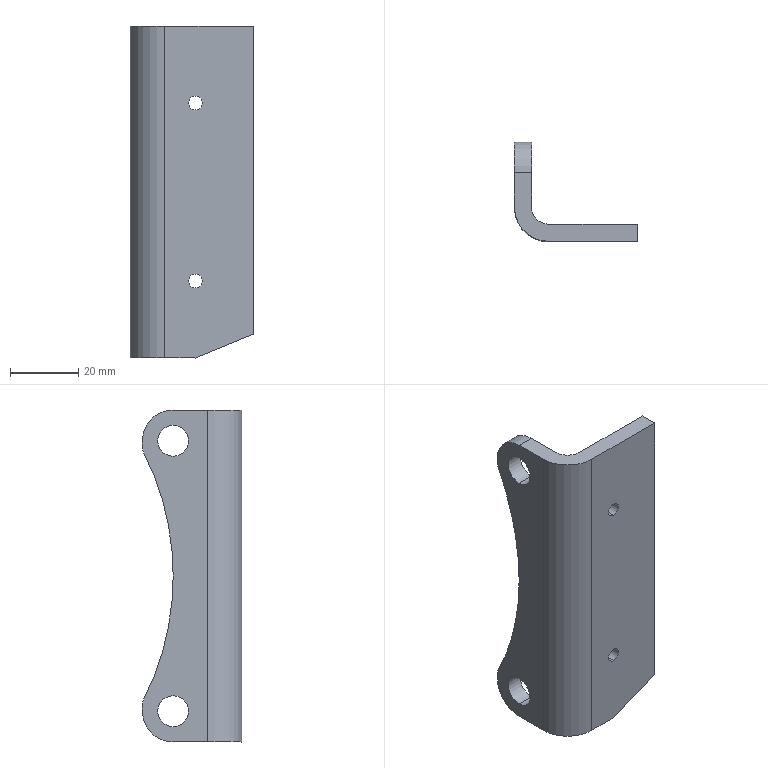Part | SolidWorks | features BaseBody 1 | 1 solid | 25 faces | box 36 x 29 x 97 mm | volume 24067 mm3 | cylinder 15 | plane 10 | commonest cylinder face diameters 4 x4 9 x4 6 x2 18 x2 10 x1 20 x1
STEP:
#1=CARTESIAN_POINT('',(19.,0.,20.5));
#2=VERTEX_POINT('',#1);
#3=CARTESIAN_POINT('',(19.,0.,24.5));
#4=VERTEX_POINT('',#3);
#5=CARTESIAN_POINT('',(19.,0.,22.5));
#6=DIRECTION('',(0.,1.,0.));
#7=DIRECTION('',(0.,0.,1.));
#8=AXIS2_PLACEMENT_3D('',#5,#6,#7);
#9=CIRCLE('',#8,2.);
#10=EDGE_CURVE('',#2,#4,#9,.T.);
#11=ORIENTED_EDGE('',*,*,#10,.F.);
#12=CARTESIAN_POINT('',(19.,5.,20.5));
#13=VERTEX_POINT('',#12);
#14=CARTESIAN_POINT('',(19.,0.,20.5));
#15=DIRECTION('',(0.,1.,0.));
#16=VECTOR('',#15,1000.);
#17=LINE('',#14,#16);
#18=EDGE_CURVE('',#2,#13,#17,.T.);
#19=ORIENTED_EDGE('',*,*,#18,.T.);
#20=CARTESIAN_POINT('',(19.,5.,24.5));
#21=VERTEX_POINT('',#20);
#22=CARTESIAN_POINT('',(19.,5.,22.5));
#23=DIRECTION('',(0.,-1.,0.));
#24=DIRECTION('',(0.,0.,1.));
#25=AXIS2_PLACEMENT_3D('',#22,#23,#24);
#26=CIRCLE('',#25,2.);
#27=EDGE_CURVE('',#21,#13,#26,.T.);
#28=ORIENTED_EDGE('',*,*,#27,.F.);
#29=CARTESIAN_POINT('',(19.,0.,24.5));
#30=DIRECTION('',(0.,1.,0.));
#31=VECTOR('',#30,1000.);
#32=LINE('',#29,#31);
#33=EDGE_CURVE('',#4,#21,#32,.T.);
#34=ORIENTED_EDGE('',*,*,#33,.F.);
#35=EDGE_LOOP('',(#11,#19,#28,#34));
#36=FACE_OUTER_BOUND('',#35,.T.);
#37=CARTESIAN_POINT('',(19.,0.,22.5));
#38=DIRECTION('',(0.,1.,0.));
#39=DIRECTION('',(0.,0.,1.));
#40=AXIS2_PLACEMENT_3D('',#37,#38,#39);
#41=CYLINDRICAL_SURFACE('',#40,2.);
#42=ADVANCED_FACE('',(#36),#41,.F.);
#43=CARTESIAN_POINT('',(19.,0.,72.5));
#44=VERTEX_POINT('',#43);
#45=CARTESIAN_POINT('',(19.,0.,76.5));
#46=VERTEX_POINT('',#45);
#47=CARTESIAN_POINT('',(19.,0.,74.5));
#48=DIRECTION('',(0.,1.,0.));
#49=DIRECTION('',(0.,0.,1.));
#50=AXIS2_PLACEMENT_3D('',#47,#48,#49);
#51=CIRCLE('',#50,2.);
#52=EDGE_CURVE('',#44,#46,#51,.T.);
#53=ORIENTED_EDGE('',*,*,#52,.F.);
#54=CARTESIAN_POINT('',(19.,5.,72.5));
#55=VERTEX_POINT('',#54);
#56=CARTESIAN_POINT('',(19.,0.,72.5));
#57=DIRECTION('',(0.,1.,0.));
#58=VECTOR('',#57,1000.);
#59=LINE('',#56,#58);
#60=EDGE_CURVE('',#44,#55,#59,.T.);
#61=ORIENTED_EDGE('',*,*,#60,.T.);
#62=CARTESIAN_POINT('',(19.,5.,76.5));
#63=VERTEX_POINT('',#62);
#64=CARTESIAN_POINT('',(19.,5.,74.5));
#65=DIRECTION('',(0.,-1.,0.));
#66=DIRECTION('',(0.,0.,1.));
#67=AXIS2_PLACEMENT_3D('',#64,#65,#66);
#68=CIRCLE('',#67,2.);
#69=EDGE_CURVE('',#63,#55,#68,.T.);
#70=ORIENTED_EDGE('',*,*,#69,.F.);
#71=CARTESIAN_POINT('',(19.,0.,76.5));
#72=DIRECTION('',(0.,1.,0.));
#73=VECTOR('',#72,1000.);
#74=LINE('',#71,#73);
#75=EDGE_CURVE('',#46,#63,#74,.T.);
#76=ORIENTED_EDGE('',*,*,#75,.F.);
#77=EDGE_LOOP('',(#53,#61,#70,#76));
#78=FACE_OUTER_BOUND('',#77,.T.);
#79=CARTESIAN_POINT('',(19.,0.,74.5));
#80=DIRECTION('',(0.,1.,0.));
#81=DIRECTION('',(0.,0.,1.));
#82=AXIS2_PLACEMENT_3D('',#79,#80,#81);
#83=CYLINDRICAL_SURFACE('',#82,2.);
#84=ADVANCED_FACE('',(#78),#83,.F.);
#85=CARTESIAN_POINT('',(0.,20.,4.5));
#86=VERTEX_POINT('',#85);
#87=CARTESIAN_POINT('',(0.,20.,13.5));
#88=VERTEX_POINT('',#87);
#89=CARTESIAN_POINT('',(0.,20.,9.));
#90=DIRECTION('',(-1.,0.,0.));
#91=DIRECTION('',(0.,0.,-1.));
#92=AXIS2_PLACEMENT_3D('',#89,#90,#91);
#93=CIRCLE('',#92,4.5);
#94=EDGE_CURVE('',#86,#88,#93,.T.);
#95=ORIENTED_EDGE('',*,*,#94,.T.);
#96=CARTESIAN_POINT('',(5.,20.,13.5));
#97=VERTEX_POINT('',#96);
#98=CARTESIAN_POINT('',(0.,20.,13.5));
#99=DIRECTION('',(1.,0.,0.));
#100=VECTOR('',#99,1000.);
#101=LINE('',#98,#100);
#102=EDGE_CURVE('',#88,#97,#101,.T.);
#103=ORIENTED_EDGE('',*,*,#102,.T.);
#104=CARTESIAN_POINT('',(5.,20.,4.5));
#105=VERTEX_POINT('',#104);
#106=CARTESIAN_POINT('',(5.,20.,9.));
#107=DIRECTION('',(-1.,0.,0.));
#108=DIRECTION('',(0.,0.,-1.));
#109=AXIS2_PLACEMENT_3D('',#106,#107,#108);
#110=CIRCLE('',#109,4.5);
#111=EDGE_CURVE('',#105,#97,#110,.T.);
#112=ORIENTED_EDGE('',*,*,#111,.F.);
#113=CARTESIAN_POINT('',(0.,20.,4.5));
#114=DIRECTION('',(1.,0.,0.));
#115=VECTOR('',#114,1000.);
#116=LINE('',#113,#115);
#117=EDGE_CURVE('',#86,#105,#116,.T.);
#118=ORIENTED_EDGE('',*,*,#117,.F.);
#119=EDGE_LOOP('',(#95,#103,#112,#118));
#120=FACE_OUTER_BOUND('',#119,.T.);
#121=CARTESIAN_POINT('',(0.,20.,9.));
#122=DIRECTION('',(1.,0.,0.));
#123=DIRECTION('',(0.,0.,-1.));
#124=AXIS2_PLACEMENT_3D('',#121,#122,#123);
#125=CYLINDRICAL_SURFACE('',#124,4.5);
#126=ADVANCED_FACE('',(#120),#125,.F.);
#127=CARTESIAN_POINT('',(0.,20.,83.5));
#128=VERTEX_POINT('',#127);
#129=CARTESIAN_POINT('',(0.,20.,92.5));
#130=VERTEX_POINT('',#129);
#131=CARTESIAN_POINT('',(0.,20.,88.));
#132=DIRECTION('',(-1.,0.,0.));
#133=DIRECTION('',(0.,0.,-1.));
#134=AXIS2_PLACEMENT_3D('',#131,#132,#133);
#135=CIRCLE('',#134,4.5);
#136=EDGE_CURVE('',#128,#130,#135,.T.);
#137=ORIENTED_EDGE('',*,*,#136,.T.);
#138=CARTESIAN_POINT('',(5.,20.,92.5));
#139=VERTEX_POINT('',#138);
#140=CARTESIAN_POINT('',(0.,20.,92.5));
#141=DIRECTION('',(1.,0.,0.));
#142=VECTOR('',#141,1000.);
#143=LINE('',#140,#142);
#144=EDGE_CURVE('',#130,#139,#143,.T.);
#145=ORIENTED_EDGE('',*,*,#144,.T.);
#146=CARTESIAN_POINT('',(5.,20.,83.5));
#147=VERTEX_POINT('',#146);
#148=CARTESIAN_POINT('',(5.,20.,88.));
#149=DIRECTION('',(-1.,0.,0.));
#150=DIRECTION('',(0.,0.,-1.));
#151=AXIS2_PLACEMENT_3D('',#148,#149,#150);
#152=CIRCLE('',#151,4.5);
#153=EDGE_CURVE('',#147,#139,#152,.T.);
#154=ORIENTED_EDGE('',*,*,#153,.F.);
#155=CARTESIAN_POINT('',(0.,20.,83.5));
#156=DIRECTION('',(1.,0.,0.));
#157=VECTOR('',#156,1000.);
#158=LINE('',#155,#157);
#159=EDGE_CURVE('',#128,#147,#158,.T.);
#160=ORIENTED_EDGE('',*,*,#159,.F.);
#161=EDGE_LOOP('',(#137,#145,#154,#160));
#162=FACE_OUTER_BOUND('',#161,.T.);
#163=CARTESIAN_POINT('',(0.,20.,88.));
#164=DIRECTION('',(1.,0.,0.));
#165=DIRECTION('',(0.,0.,-1.));
#166=AXIS2_PLACEMENT_3D('',#163,#164,#165);
#167=CYLINDRICAL_SURFACE('',#166,4.5);
#168=ADVANCED_FACE('',(#162),#167,.F.);
#169=ORIENTED_EDGE('',*,*,#27,.T.);
#170=CARTESIAN_POINT('',(19.,5.,22.5));
#171=DIRECTION('',(0.,-1.,0.));
#172=DIRECTION('',(0.,0.,1.));
#173=AXIS2_PLACEMENT_3D('',#170,#171,#172);
#174=CIRCLE('',#173,2.);
#175=EDGE_CURVE('',#13,#21,#174,.T.);
#176=ORIENTED_EDGE('',*,*,#175,.T.);
#177=EDGE_LOOP('',(#169,#176));
#178=FACE_BOUND('',#177,.T.);
#179=ORIENTED_EDGE('',*,*,#69,.T.);
#180=CARTESIAN_POINT('',(19.,5.,74.5));
#181=DIRECTION('',(0.,-1.,0.));
#182=DIRECTION('',(0.,0.,1.));
#183=AXIS2_PLACEMENT_3D('',#180,#181,#182);
#184=CIRCLE('',#183,2.);
#185=EDGE_CURVE('',#55,#63,#184,.T.);
#186=ORIENTED_EDGE('',*,*,#185,.T.);
#187=EDGE_LOOP('',(#179,#186));
#188=FACE_BOUND('',#187,.T.);
#189=CARTESIAN_POINT('',(10.,5.,97.));
#190=VERTEX_POINT('',#189);
#191=CARTESIAN_POINT('',(36.,5.,97.));
#192=VERTEX_POINT('',#191);
#193=CARTESIAN_POINT('',(23.,5.,97.));
#194=DIRECTION('',(1.,0.,0.));
#195=VECTOR('',#194,1000.);
#196=LINE('',#193,#195);
#197=EDGE_CURVE('',#190,#192,#196,.T.);
#198=ORIENTED_EDGE('',*,*,#197,.T.);
#199=CARTESIAN_POINT('',(36.,5.,7.));
#200=VERTEX_POINT('',#199);
#201=CARTESIAN_POINT('',(36.,5.,48.5));
#202=DIRECTION('',(0.,0.,-1.));
#203=VECTOR('',#202,1000.);
#204=LINE('',#201,#203);
#205=EDGE_CURVE('',#192,#200,#204,.T.);
#206=ORIENTED_EDGE('',*,*,#205,.T.);
#207=CARTESIAN_POINT('',(19.,5.,0.));
#208=VERTEX_POINT('',#207);
#209=CARTESIAN_POINT('',(36.,5.,7.));
#210=DIRECTION('',(-0.9247,0.,-0.3807));
#211=VECTOR('',#210,1000.);
#212=LINE('',#209,#211);
#213=EDGE_CURVE('',#200,#208,#212,.T.);
#214=ORIENTED_EDGE('',*,*,#213,.T.);
#215=CARTESIAN_POINT('',(10.,5.,0.));
#216=VERTEX_POINT('',#215);
#217=CARTESIAN_POINT('',(23.,5.,0.));
#218=DIRECTION('',(-1.,0.,0.));
#219=VECTOR('',#218,1000.);
#220=LINE('',#217,#219);
#221=EDGE_CURVE('',#208,#216,#220,.T.);
#222=ORIENTED_EDGE('',*,*,#221,.T.);
#223=CARTESIAN_POINT('',(10.,5.,48.5));
#224=DIRECTION('',(0.,0.,1.));
#225=VECTOR('',#224,1000.);
#226=LINE('',#223,#225);
#227=EDGE_CURVE('',#216,#190,#226,.T.);
#228=ORIENTED_EDGE('',*,*,#227,.T.);
#229=EDGE_LOOP('',(#198,#206,#214,#222,#228));
#230=FACE_OUTER_BOUND('',#229,.T.);
#231=CARTESIAN_POINT('',(23.,5.,48.5));
#232=DIRECTION('',(0.,1.,0.));
#233=DIRECTION('',(0.,0.,1.));
#234=AXIS2_PLACEMENT_3D('',#231,#232,#233);
#235=PLANE('',#234);
#236=ADVANCED_FACE('',(#178,#188,#230),#235,.T.);
#237=ORIENTED_EDGE('',*,*,#18,.F.);
#238=CARTESIAN_POINT('',(19.,0.,22.5));
#239=DIRECTION('',(0.,1.,0.));
#240=DIRECTION('',(0.,0.,1.));
#241=AXIS2_PLACEMENT_3D('',#238,#239,#240);
#242=CIRCLE('',#241,2.);
#243=EDGE_CURVE('',#4,#2,#242,.T.);
#244=ORIENTED_EDGE('',*,*,#243,.F.);
#245=ORIENTED_EDGE('',*,*,#33,.T.);
#246=ORIENTED_EDGE('',*,*,#175,.F.);
#247=EDGE_LOOP('',(#237,#244,#245,#246));
#248=FACE_OUTER_BOUND('',#247,.T.);
#249=CARTESIAN_POINT('',(19.,0.,22.5));
#250=DIRECTION('',(0.,1.,0.));
#251=DIRECTION('',(0.,0.,1.));
#252=AXIS2_PLACEMENT_3D('',#249,#250,#251);
#253=CYLINDRICAL_SURFACE('',#252,2.);
#254=ADVANCED_FACE('',(#248),#253,.F.);
#255=ORIENTED_EDGE('',*,*,#60,.F.);
#256=CARTESIAN_POINT('',(19.,0.,74.5));
#257=DIRECTION('',(0.,1.,0.));
#258=DIRECTION('',(0.,0.,1.));
#259=AXIS2_PLACEMENT_3D('',#256,#257,#258);
#260=CIRCLE('',#259,2.);
#261=EDGE_CURVE('',#46,#44,#260,.T.);
#262=ORIENTED_EDGE('',*,*,#261,.F.);
#263=ORIENTED_EDGE('',*,*,#75,.T.);
#264=ORIENTED_EDGE('',*,*,#185,.F.);
#265=EDGE_LOOP('',(#255,#262,#263,#264));
#266=FACE_OUTER_BOUND('',#265,.T.);
#267=CARTESIAN_POINT('',(19.,0.,74.5));
#268=DIRECTION('',(0.,1.,0.));
#269=DIRECTION('',(0.,0.,1.));
#270=AXIS2_PLACEMENT_3D('',#267,#268,#269);
#271=CYLINDRICAL_SURFACE('',#270,2.);
#272=ADVANCED_FACE('',(#266),#271,.F.);
#273=CARTESIAN_POINT('',(36.,0.,97.));
#274=VERTEX_POINT('',#273);
#275=CARTESIAN_POINT('',(36.,2.5,97.));
#276=DIRECTION('',(0.,-1.,0.));
#277=VECTOR('',#276,1000.);
#278=LINE('',#275,#277);
#279=EDGE_CURVE('',#192,#274,#278,.T.);
#280=ORIENTED_EDGE('',*,*,#279,.T.);
#281=CARTESIAN_POINT('',(36.,0.,7.));
#282=VERTEX_POINT('',#281);
#283=CARTESIAN_POINT('',(36.,0.,52.));
#284=DIRECTION('',(0.,0.,-1.));
#285=VECTOR('',#284,1000.);
#286=LINE('',#283,#285);
#287=EDGE_CURVE('',#274,#282,#286,.T.);
#288=ORIENTED_EDGE('',*,*,#287,.T.);
#289=CARTESIAN_POINT('',(36.,2.5,7.));
#290=DIRECTION('',(0.,1.,0.));
#291=VECTOR('',#290,1000.);
#292=LINE('',#289,#291);
#293=EDGE_CURVE('',#282,#200,#292,.T.);
#294=ORIENTED_EDGE('',*,*,#293,.T.);
#295=ORIENTED_EDGE('',*,*,#205,.F.);
#296=EDGE_LOOP('',(#280,#288,#294,#295));
#297=FACE_OUTER_BOUND('',#296,.T.);
#298=CARTESIAN_POINT('',(36.,2.5,52.));
#299=DIRECTION('',(1.,0.,0.));
#300=DIRECTION('',(0.,0.,-1.));
#301=AXIS2_PLACEMENT_3D('',#298,#299,#300);
#302=PLANE('',#301);
#303=ADVANCED_FACE('',(#297),#302,.T.);
#304=CARTESIAN_POINT('',(5.,10.,97.));
#305=VERTEX_POINT('',#304);
#306=CARTESIAN_POINT('',(10.,10.,97.));
#307=DIRECTION('',(0.,0.,-1.));
#308=DIRECTION('',(-1.,0.,0.));
#309=AXIS2_PLACEMENT_3D('',#306,#307,#308);
#310=CIRCLE('',#309,5.);
#311=EDGE_CURVE('',#190,#305,#310,.T.);
#312=ORIENTED_EDGE('',*,*,#311,.T.);
#313=CARTESIAN_POINT('',(5.,20.,97.));
#314=VERTEX_POINT('',#313);
#315=CARTESIAN_POINT('',(5.,10.,97.));
#316=DIRECTION('',(0.,1.,0.));
#317=VECTOR('',#316,1000.);
#318=LINE('',#315,#317);
#319=EDGE_CURVE('',#305,#314,#318,.T.);
#320=ORIENTED_EDGE('',*,*,#319,.T.);
#321=CARTESIAN_POINT('',(0.,20.,97.));
#322=VERTEX_POINT('',#321);
#323=CARTESIAN_POINT('',(18.,20.,97.));
#324=DIRECTION('',(-1.,0.,0.));
#325=VECTOR('',#324,1000.);
#326=LINE('',#323,#325);
#327=EDGE_CURVE('',#314,#322,#326,.T.);
#328=ORIENTED_EDGE('',*,*,#327,.T.);
#329=CARTESIAN_POINT('',(0.,10.,97.));
#330=VERTEX_POINT('',#329);
#331=CARTESIAN_POINT('',(0.,10.,97.));
#332=DIRECTION('',(0.,-1.,0.));
#333=VECTOR('',#332,1000.);
#334=LINE('',#331,#333);
#335=EDGE_CURVE('',#322,#330,#334,.T.);
#336=ORIENTED_EDGE('',*,*,#335,.T.);
#337=CARTESIAN_POINT('',(10.,0.,97.));
#338=VERTEX_POINT('',#337);
#339=CARTESIAN_POINT('',(10.,10.,97.));
#340=DIRECTION('',(0.,0.,1.));
#341=DIRECTION('',(-1.,0.,0.));
#342=AXIS2_PLACEMENT_3D('',#339,#340,#341);
#343=CIRCLE('',#342,10.);
#344=EDGE_CURVE('',#330,#338,#343,.T.);
#345=ORIENTED_EDGE('',*,*,#344,.T.);
#346=CARTESIAN_POINT('',(18.,0.,97.));
#347=DIRECTION('',(1.,0.,0.));
#348=VECTOR('',#347,1000.);
#349=LINE('',#346,#348);
#350=EDGE_CURVE('',#338,#274,#349,.T.);
#351=ORIENTED_EDGE('',*,*,#350,.T.);
#352=ORIENTED_EDGE('',*,*,#279,.F.);
#353=ORIENTED_EDGE('',*,*,#197,.F.);
#354=EDGE_LOOP('',(#312,#320,#328,#336,#345,#351,#352,#353));
#355=FACE_OUTER_BOUND('',#354,.T.);
#356=CARTESIAN_POINT('',(18.,10.,97.));
#357=DIRECTION('',(0.,0.,1.));
#358=DIRECTION('',(1.,0.,0.));
#359=AXIS2_PLACEMENT_3D('',#356,#357,#358);
#360=PLANE('',#359);
#361=ADVANCED_FACE('',(#355),#360,.T.);
#362=ORIENTED_EDGE('',*,*,#227,.F.);
#363=CARTESIAN_POINT('',(5.,10.,0.));
#364=VERTEX_POINT('',#363);
#365=CARTESIAN_POINT('',(10.,10.,0.));
#366=DIRECTION('',(0.,0.,1.));
#367=DIRECTION('',(-1.,0.,0.));
#368=AXIS2_PLACEMENT_3D('',#365,#366,#367);
#369=CIRCLE('',#368,5.);
#370=EDGE_CURVE('',#364,#216,#369,.T.);
#371=ORIENTED_EDGE('',*,*,#370,.F.);
#372=CARTESIAN_POINT('',(5.,10.,97.));
#373=DIRECTION('',(0.,0.,-1.));
#374=VECTOR('',#373,1000.);
#375=LINE('',#372,#374);
#376=EDGE_CURVE('',#305,#364,#375,.T.);
#377=ORIENTED_EDGE('',*,*,#376,.F.);
#378=ORIENTED_EDGE('',*,*,#311,.F.);
#379=EDGE_LOOP('',(#362,#371,#377,#378));
#380=FACE_OUTER_BOUND('',#379,.T.);
#381=CARTESIAN_POINT('',(10.,10.,97.));
#382=DIRECTION('',(0.,0.,-1.));
#383=DIRECTION('',(-1.,0.,0.));
#384=AXIS2_PLACEMENT_3D('',#381,#382,#383);
#385=CYLINDRICAL_SURFACE('',#384,5.);
#386=ADVANCED_FACE('',(#380),#385,.F.);
#387=CARTESIAN_POINT('',(19.,0.,0.));
#388=VERTEX_POINT('',#387);
#389=CARTESIAN_POINT('',(19.,10.,0.));
#390=DIRECTION('',(0.,1.,0.));
#391=VECTOR('',#390,1000.);
#392=LINE('',#389,#391);
#393=EDGE_CURVE('',#388,#208,#392,.T.);
#394=ORIENTED_EDGE('',*,*,#393,.F.);
#395=CARTESIAN_POINT('',(10.,0.,0.));
#396=VERTEX_POINT('',#395);
#397=CARTESIAN_POINT('',(9.5,0.,0.));
#398=DIRECTION('',(1.,0.,0.));
#399=VECTOR('',#398,1000.);
#400=LINE('',#397,#399);
#401=EDGE_CURVE('',#396,#388,#400,.T.);
#402=ORIENTED_EDGE('',*,*,#401,.F.);
#403=CARTESIAN_POINT('',(0.,10.,0.));
#404=VERTEX_POINT('',#403);
#405=CARTESIAN_POINT('',(10.,10.,0.));
#406=DIRECTION('',(0.,0.,1.));
#407=DIRECTION('',(-1.,0.,0.));
#408=AXIS2_PLACEMENT_3D('',#405,#406,#407);
#409=CIRCLE('',#408,10.);
#410=EDGE_CURVE('',#404,#396,#409,.T.);
#411=ORIENTED_EDGE('',*,*,#410,.F.);
#412=CARTESIAN_POINT('',(0.,20.,0.));
#413=VERTEX_POINT('',#412);
#414=CARTESIAN_POINT('',(0.,10.,0.));
#415=DIRECTION('',(0.,-1.,0.));
#416=VECTOR('',#415,1000.);
#417=LINE('',#414,#416);
#418=EDGE_CURVE('',#413,#404,#417,.T.);
#419=ORIENTED_EDGE('',*,*,#418,.F.);
#420=CARTESIAN_POINT('',(5.,20.,0.));
#421=VERTEX_POINT('',#420);
#422=CARTESIAN_POINT('',(9.5,20.,0.));
#423=DIRECTION('',(-1.,0.,0.));
#424=VECTOR('',#423,1000.);
#425=LINE('',#422,#424);
#426=EDGE_CURVE('',#421,#413,#425,.T.);
#427=ORIENTED_EDGE('',*,*,#426,.F.);
#428=CARTESIAN_POINT('',(5.,10.,0.));
#429=DIRECTION('',(0.,1.,0.));
#430=VECTOR('',#429,1000.);
#431=LINE('',#428,#430);
#432=EDGE_CURVE('',#364,#421,#431,.T.);
#433=ORIENTED_EDGE('',*,*,#432,.F.);
#434=ORIENTED_EDGE('',*,*,#370,.T.);
#435=ORIENTED_EDGE('',*,*,#221,.F.);
#436=EDGE_LOOP('',(#394,#402,#411,#419,#427,#433,#434,#435));
#437=FACE_OUTER_BOUND('',#436,.T.);
#438=CARTESIAN_POINT('',(9.5,10.,0.));
#439=DIRECTION('',(0.,0.,1.));
#440=DIRECTION('',(1.,0.,0.));
#441=AXIS2_PLACEMENT_3D('',#438,#439,#440);
#442=PLANE('',#441);
#443=ADVANCED_FACE('',(#437),#442,.F.);
#444=ORIENTED_EDGE('',*,*,#213,.F.);
#445=ORIENTED_EDGE('',*,*,#293,.F.);
#446=CARTESIAN_POINT('',(27.5,0.,3.5));
#447=DIRECTION('',(0.9247,0.,0.3807));
#448=VECTOR('',#447,1000.);
#449=LINE('',#446,#448);
#450=EDGE_CURVE('',#388,#282,#449,.T.);
#451=ORIENTED_EDGE('',*,*,#450,.F.);
#452=ORIENTED_EDGE('',*,*,#393,.T.);
#453=EDGE_LOOP('',(#444,#445,#451,#452));
#454=FACE_OUTER_BOUND('',#453,.T.);
#455=CARTESIAN_POINT('',(27.5,2.5,3.5));
#456=DIRECTION('',(-0.3807,0.,0.9247));
#457=DIRECTION('',(0.9247,0.,0.3807));
#458=AXIS2_PLACEMENT_3D('',#455,#456,#457);
#459=PLANE('',#458);
#460=ADVANCED_FACE('',(#454),#459,.F.);
#461=ORIENTED_EDGE('',*,*,#243,.T.);
#462=ORIENTED_EDGE('',*,*,#10,.T.);
#463=EDGE_LOOP('',(#461,#462));
#464=FACE_BOUND('',#463,.T.);
#465=ORIENTED_EDGE('',*,*,#261,.T.);
#466=ORIENTED_EDGE('',*,*,#52,.T.);
#467=EDGE_LOOP('',(#465,#466));
#468=FACE_BOUND('',#467,.T.);
#469=ORIENTED_EDGE('',*,*,#287,.F.);
#470=ORIENTED_EDGE('',*,*,#350,.F.);
#471=CARTESIAN_POINT('',(10.,0.,48.5));
#472=DIRECTION('',(0.,0.,1.));
#473=VECTOR('',#472,1000.);
#474=LINE('',#471,#473);
#475=EDGE_CURVE('',#396,#338,#474,.T.);
#476=ORIENTED_EDGE('',*,*,#475,.F.);
#477=ORIENTED_EDGE('',*,*,#401,.T.);
#478=ORIENTED_EDGE('',*,*,#450,.T.);
#479=EDGE_LOOP('',(#469,#470,#476,#477,#478));
#480=FACE_OUTER_BOUND('',#479,.T.);
#481=CARTESIAN_POINT('',(23.,0.,48.5));
#482=DIRECTION('',(0.,1.,0.));
#483=DIRECTION('',(0.,0.,1.));
#484=AXIS2_PLACEMENT_3D('',#481,#482,#483);
#485=PLANE('',#484);
#486=ADVANCED_FACE('',(#464,#468,#480),#485,.F.);
#487=ORIENTED_EDGE('',*,*,#111,.T.);
#488=CARTESIAN_POINT('',(5.,20.,9.));
#489=DIRECTION('',(-1.,0.,0.));
#490=DIRECTION('',(0.,0.,-1.));
#491=AXIS2_PLACEMENT_3D('',#488,#489,#490);
#492=CIRCLE('',#491,4.5);
#493=EDGE_CURVE('',#97,#105,#492,.T.);
#494=ORIENTED_EDGE('',*,*,#493,.T.);
#495=EDGE_LOOP('',(#487,#494));
#496=FACE_BOUND('',#495,.T.);
#497=ORIENTED_EDGE('',*,*,#153,.T.);
#498=CARTESIAN_POINT('',(5.,20.,88.));
#499=DIRECTION('',(-1.,0.,0.));
#500=DIRECTION('',(0.,0.,-1.));
#501=AXIS2_PLACEMENT_3D('',#498,#499,#500);
#502=CIRCLE('',#501,4.5);
#503=EDGE_CURVE('',#139,#147,#502,.T.);
#504=ORIENTED_EDGE('',*,*,#503,.T.);
#505=EDGE_LOOP('',(#497,#504));
#506=FACE_BOUND('',#505,.T.);
#507=CARTESIAN_POINT('',(5.,29.,9.));
#508=VERTEX_POINT('',#507);
#509=CARTESIAN_POINT('',(5.,20.,9.));
#510=DIRECTION('',(1.,0.,0.));
#511=DIRECTION('',(0.,0.,-1.));
#512=AXIS2_PLACEMENT_3D('',#509,#510,#511);
#513=CIRCLE('',#512,9.);
#514=EDGE_CURVE('',#421,#508,#513,.T.);
#515=ORIENTED_EDGE('',*,*,#514,.T.);
#516=CARTESIAN_POINT('',(5.,29.,10.91));
#517=VERTEX_POINT('',#516);
#518=CARTESIAN_POINT('',(5.,29.,48.5));
#519=DIRECTION('',(0.,0.,1.));
#520=VECTOR('',#519,1000.);
#521=LINE('',#518,#520);
#522=EDGE_CURVE('',#508,#517,#521,.T.);
#523=ORIENTED_EDGE('',*,*,#522,.T.);
#524=CARTESIAN_POINT('',(5.,28.675,12.269));
#525=VERTEX_POINT('',#524);
#526=CARTESIAN_POINT('',(5.,26.,10.91));
#527=DIRECTION('',(-1.,0.,0.));
#528=DIRECTION('',(0.,0.,-1.));
#529=AXIS2_PLACEMENT_3D('',#526,#527,#528);
#530=CIRCLE('',#529,3.);
#531=EDGE_CURVE('',#525,#517,#530,.T.);
#532=ORIENTED_EDGE('',*,*,#531,.F.);
#533=CARTESIAN_POINT('',(5.,28.675,84.731));
#534=VERTEX_POINT('',#533);
#535=CARTESIAN_POINT('',(5.,100.,48.5));
#536=DIRECTION('',(-1.,0.,0.));
#537=DIRECTION('',(0.,0.,-1.));
#538=AXIS2_PLACEMENT_3D('',#535,#536,#537);
#539=CIRCLE('',#538,80.);
#540=EDGE_CURVE('',#525,#534,#539,.T.);
#541=ORIENTED_EDGE('',*,*,#540,.T.);
#542=CARTESIAN_POINT('',(5.,29.,86.09));
#543=VERTEX_POINT('',#542);
#544=CARTESIAN_POINT('',(5.,26.,86.09));
#545=DIRECTION('',(-1.,0.,0.));
#546=DIRECTION('',(0.,0.,-1.));
#547=AXIS2_PLACEMENT_3D('',#544,#545,#546);
#548=CIRCLE('',#547,3.);
#549=EDGE_CURVE('',#543,#534,#548,.T.);
#550=ORIENTED_EDGE('',*,*,#549,.F.);
#551=CARTESIAN_POINT('',(5.,29.,88.));
#552=VERTEX_POINT('',#551);
#553=CARTESIAN_POINT('',(5.,29.,48.5));
#554=DIRECTION('',(0.,0.,1.));
#555=VECTOR('',#554,1000.);
#556=LINE('',#553,#555);
#557=EDGE_CURVE('',#543,#552,#556,.T.);
#558=ORIENTED_EDGE('',*,*,#557,.T.);
#559=CARTESIAN_POINT('',(5.,20.,88.));
#560=DIRECTION('',(1.,0.,0.));
#561=DIRECTION('',(0.,0.,-1.));
#562=AXIS2_PLACEMENT_3D('',#559,#560,#561);
#563=CIRCLE('',#562,9.);
#564=EDGE_CURVE('',#552,#314,#563,.T.);
#565=ORIENTED_EDGE('',*,*,#564,.T.);
#566=ORIENTED_EDGE('',*,*,#319,.F.);
#567=ORIENTED_EDGE('',*,*,#376,.T.);
#568=ORIENTED_EDGE('',*,*,#432,.T.);
#569=EDGE_LOOP('',(#515,#523,#532,#541,#550,#558,#565,#566,#567,#568));
#570=FACE_OUTER_BOUND('',#569,.T.);
#571=CARTESIAN_POINT('',(5.,19.5,48.5));
#572=DIRECTION('',(1.,0.,0.));
#573=DIRECTION('',(0.,0.,-1.));
#574=AXIS2_PLACEMENT_3D('',#571,#572,#573);
#575=PLANE('',#574);
#576=ADVANCED_FACE('',(#496,#506,#570),#575,.T.);
#577=ORIENTED_EDGE('',*,*,#410,.T.);
#578=ORIENTED_EDGE('',*,*,#475,.T.);
#579=ORIENTED_EDGE('',*,*,#344,.F.);
#580=CARTESIAN_POINT('',(0.,10.,97.));
#581=DIRECTION('',(0.,0.,-1.));
#582=VECTOR('',#581,1000.);
#583=LINE('',#580,#582);
#584=EDGE_CURVE('',#330,#404,#583,.T.);
#585=ORIENTED_EDGE('',*,*,#584,.T.);
#586=EDGE_LOOP('',(#577,#578,#579,#585));
#587=FACE_OUTER_BOUND('',#586,.T.);
#588=CARTESIAN_POINT('',(10.,10.,97.));
#589=DIRECTION('',(0.,0.,-1.));
#590=DIRECTION('',(-1.,0.,0.));
#591=AXIS2_PLACEMENT_3D('',#588,#589,#590);
#592=CYLINDRICAL_SURFACE('',#591,10.);
#593=ADVANCED_FACE('',(#587),#592,.T.);
#594=ORIENTED_EDGE('',*,*,#94,.F.);
#595=CARTESIAN_POINT('',(0.,20.,9.));
#596=DIRECTION('',(-1.,0.,0.));
#597=DIRECTION('',(0.,0.,-1.));
#598=AXIS2_PLACEMENT_3D('',#595,#596,#597);
#599=CIRCLE('',#598,4.5);
#600=EDGE_CURVE('',#88,#86,#599,.T.);
#601=ORIENTED_EDGE('',*,*,#600,.F.);
#602=EDGE_LOOP('',(#594,#601));
#603=FACE_BOUND('',#602,.T.);
#604=ORIENTED_EDGE('',*,*,#136,.F.);
#605=CARTESIAN_POINT('',(0.,20.,88.));
#606=DIRECTION('',(-1.,0.,0.));
#607=DIRECTION('',(0.,0.,-1.));
#608=AXIS2_PLACEMENT_3D('',#605,#606,#607);
#609=CIRCLE('',#608,4.5);
#610=EDGE_CURVE('',#130,#128,#609,.T.);
#611=ORIENTED_EDGE('',*,*,#610,.F.);
#612=EDGE_LOOP('',(#604,#611));
#613=FACE_BOUND('',#612,.T.);
#614=CARTESIAN_POINT('',(0.,29.,9.));
#615=VERTEX_POINT('',#614);
#616=CARTESIAN_POINT('',(0.,29.,10.91));
#617=VERTEX_POINT('',#616);
#618=CARTESIAN_POINT('',(0.,29.,48.5));
#619=DIRECTION('',(0.,0.,1.));
#620=VECTOR('',#619,1000.);
#621=LINE('',#618,#620);
#622=EDGE_CURVE('',#615,#617,#621,.T.);
#623=ORIENTED_EDGE('',*,*,#622,.F.);
#624=CARTESIAN_POINT('',(0.,20.,9.));
#625=DIRECTION('',(1.,0.,0.));
#626=DIRECTION('',(0.,0.,-1.));
#627=AXIS2_PLACEMENT_3D('',#624,#625,#626);
#628=CIRCLE('',#627,9.);
#629=EDGE_CURVE('',#413,#615,#628,.T.);
#630=ORIENTED_EDGE('',*,*,#629,.F.);
#631=ORIENTED_EDGE('',*,*,#418,.T.);
#632=ORIENTED_EDGE('',*,*,#584,.F.);
#633=ORIENTED_EDGE('',*,*,#335,.F.);
#634=CARTESIAN_POINT('',(0.,29.,88.));
#635=VERTEX_POINT('',#634);
#636=CARTESIAN_POINT('',(0.,20.,88.));
#637=DIRECTION('',(1.,0.,0.));
#638=DIRECTION('',(0.,0.,-1.));
#639=AXIS2_PLACEMENT_3D('',#636,#637,#638);
#640=CIRCLE('',#639,9.);
#641=EDGE_CURVE('',#635,#322,#640,.T.);
#642=ORIENTED_EDGE('',*,*,#641,.F.);
#643=CARTESIAN_POINT('',(0.,29.,86.09));
#644=VERTEX_POINT('',#643);
#645=CARTESIAN_POINT('',(0.,29.,48.5));
#646=DIRECTION('',(0.,0.,1.));
#647=VECTOR('',#646,1000.);
#648=LINE('',#645,#647);
#649=EDGE_CURVE('',#644,#635,#648,.T.);
#650=ORIENTED_EDGE('',*,*,#649,.F.);
#651=CARTESIAN_POINT('',(0.,28.675,84.731));
#652=VERTEX_POINT('',#651);
#653=CARTESIAN_POINT('',(0.,26.,86.09));
#654=DIRECTION('',(1.,0.,0.));
#655=DIRECTION('',(0.,0.,-1.));
#656=AXIS2_PLACEMENT_3D('',#653,#654,#655);
#657=CIRCLE('',#656,3.);
#658=EDGE_CURVE('',#652,#644,#657,.T.);
#659=ORIENTED_EDGE('',*,*,#658,.F.);
#660=CARTESIAN_POINT('',(0.,28.675,12.269));
#661=VERTEX_POINT('',#660);
#662=CARTESIAN_POINT('',(0.,100.,48.5));
#663=DIRECTION('',(-1.,0.,0.));
#664=DIRECTION('',(0.,0.,-1.));
#665=AXIS2_PLACEMENT_3D('',#662,#663,#664);
#666=CIRCLE('',#665,80.);
#667=EDGE_CURVE('',#661,#652,#666,.T.);
#668=ORIENTED_EDGE('',*,*,#667,.F.);
#669=CARTESIAN_POINT('',(0.,26.,10.91));
#670=DIRECTION('',(1.,0.,0.));
#671=DIRECTION('',(0.,0.,-1.));
#672=AXIS2_PLACEMENT_3D('',#669,#670,#671);
#673=CIRCLE('',#672,3.);
#674=EDGE_CURVE('',#617,#661,#673,.T.);
#675=ORIENTED_EDGE('',*,*,#674,.F.);
#676=EDGE_LOOP('',(#623,#630,#631,#632,#633,#642,#650,#659,#668,#675));
#677=FACE_OUTER_BOUND('',#676,.T.);
#678=CARTESIAN_POINT('',(0.,19.5,48.5));
#679=DIRECTION('',(1.,0.,0.));
#680=DIRECTION('',(0.,0.,-1.));
#681=AXIS2_PLACEMENT_3D('',#678,#679,#680);
#682=PLANE('',#681);
#683=ADVANCED_FACE('',(#603,#613,#677),#682,.F.);
#684=ORIENTED_EDGE('',*,*,#564,.F.);
#685=CARTESIAN_POINT('',(0.,29.,88.));
#686=DIRECTION('',(-1.,0.,0.));
#687=VECTOR('',#686,1000.);
#688=LINE('',#685,#687);
#689=EDGE_CURVE('',#552,#635,#688,.T.);
#690=ORIENTED_EDGE('',*,*,#689,.T.);
#691=ORIENTED_EDGE('',*,*,#641,.T.);
#692=ORIENTED_EDGE('',*,*,#327,.F.);
#693=EDGE_LOOP('',(#684,#690,#691,#692));
#694=FACE_OUTER_BOUND('',#693,.T.);
#695=CARTESIAN_POINT('',(0.,20.,88.));
#696=DIRECTION('',(1.,0.,0.));
#697=DIRECTION('',(0.,0.,-1.));
#698=AXIS2_PLACEMENT_3D('',#695,#696,#697);
#699=CYLINDRICAL_SURFACE('',#698,9.);
#700=ADVANCED_FACE('',(#694),#699,.T.);
#701=ORIENTED_EDGE('',*,*,#514,.F.);
#702=ORIENTED_EDGE('',*,*,#426,.T.);
#703=ORIENTED_EDGE('',*,*,#629,.T.);
#704=CARTESIAN_POINT('',(0.,29.,9.));
#705=DIRECTION('',(1.,0.,0.));
#706=VECTOR('',#705,1000.);
#707=LINE('',#704,#706);
#708=EDGE_CURVE('',#615,#508,#707,.T.);
#709=ORIENTED_EDGE('',*,*,#708,.T.);
#710=EDGE_LOOP('',(#701,#702,#703,#709));
#711=FACE_OUTER_BOUND('',#710,.T.);
#712=CARTESIAN_POINT('',(0.,20.,9.));
#713=DIRECTION('',(1.,0.,0.));
#714=DIRECTION('',(0.,0.,-1.));
#715=AXIS2_PLACEMENT_3D('',#712,#713,#714);
#716=CYLINDRICAL_SURFACE('',#715,9.);
#717=ADVANCED_FACE('',(#711),#716,.T.);
#718=ORIENTED_EDGE('',*,*,#102,.F.);
#719=ORIENTED_EDGE('',*,*,#600,.T.);
#720=ORIENTED_EDGE('',*,*,#117,.T.);
#721=ORIENTED_EDGE('',*,*,#493,.F.);
#722=EDGE_LOOP('',(#718,#719,#720,#721));
#723=FACE_OUTER_BOUND('',#722,.T.);
#724=CARTESIAN_POINT('',(0.,20.,9.));
#725=DIRECTION('',(1.,0.,0.));
#726=DIRECTION('',(0.,0.,-1.));
#727=AXIS2_PLACEMENT_3D('',#724,#725,#726);
#728=CYLINDRICAL_SURFACE('',#727,4.5);
#729=ADVANCED_FACE('',(#723),#728,.F.);
#730=ORIENTED_EDGE('',*,*,#144,.F.);
#731=ORIENTED_EDGE('',*,*,#610,.T.);
#732=ORIENTED_EDGE('',*,*,#159,.T.);
#733=ORIENTED_EDGE('',*,*,#503,.F.);
#734=EDGE_LOOP('',(#730,#731,#732,#733));
#735=FACE_OUTER_BOUND('',#734,.T.);
#736=CARTESIAN_POINT('',(0.,20.,88.));
#737=DIRECTION('',(1.,0.,0.));
#738=DIRECTION('',(0.,0.,-1.));
#739=AXIS2_PLACEMENT_3D('',#736,#737,#738);
#740=CYLINDRICAL_SURFACE('',#739,4.5);
#741=ADVANCED_FACE('',(#735),#740,.F.);
#742=ORIENTED_EDGE('',*,*,#622,.T.);
#743=CARTESIAN_POINT('',(2.5,29.,10.91));
#744=DIRECTION('',(1.,0.,0.));
#745=VECTOR('',#744,1000.);
#746=LINE('',#743,#745);
#747=EDGE_CURVE('',#617,#517,#746,.T.);
#748=ORIENTED_EDGE('',*,*,#747,.T.);
#749=ORIENTED_EDGE('',*,*,#522,.F.);
#750=ORIENTED_EDGE('',*,*,#708,.F.);
#751=EDGE_LOOP('',(#742,#748,#749,#750));
#752=FACE_OUTER_BOUND('',#751,.T.);
#753=CARTESIAN_POINT('',(2.5,29.,9.955));
#754=DIRECTION('',(0.,1.,0.));
#755=DIRECTION('',(0.,0.,1.));
#756=AXIS2_PLACEMENT_3D('',#753,#754,#755);
#757=PLANE('',#756);
#758=ADVANCED_FACE('',(#752),#757,.T.);
#759=ORIENTED_EDGE('',*,*,#689,.F.);
#760=ORIENTED_EDGE('',*,*,#557,.F.);
#761=CARTESIAN_POINT('',(2.5,29.,86.09));
#762=DIRECTION('',(-1.,0.,0.));
#763=VECTOR('',#762,1000.);
#764=LINE('',#761,#763);
#765=EDGE_CURVE('',#543,#644,#764,.T.);
#766=ORIENTED_EDGE('',*,*,#765,.T.);
#767=ORIENTED_EDGE('',*,*,#649,.T.);
#768=EDGE_LOOP('',(#759,#760,#766,#767));
#769=FACE_OUTER_BOUND('',#768,.T.);
#770=CARTESIAN_POINT('',(2.5,29.,87.045));
#771=DIRECTION('',(0.,1.,0.));
#772=DIRECTION('',(0.,0.,1.));
#773=AXIS2_PLACEMENT_3D('',#770,#771,#772);
#774=PLANE('',#773);
#775=ADVANCED_FACE('',(#769),#774,.T.);
#776=CARTESIAN_POINT('',(0.,28.675,84.731));
#777=DIRECTION('',(-1.,0.,0.));
#778=VECTOR('',#777,1000.);
#779=LINE('',#776,#778);
#780=EDGE_CURVE('',#534,#652,#779,.T.);
#781=ORIENTED_EDGE('',*,*,#780,.F.);
#782=ORIENTED_EDGE('',*,*,#540,.F.);
#783=CARTESIAN_POINT('',(0.,28.675,12.269));
#784=DIRECTION('',(1.,0.,0.));
#785=VECTOR('',#784,1000.);
#786=LINE('',#783,#785);
#787=EDGE_CURVE('',#661,#525,#786,.T.);
#788=ORIENTED_EDGE('',*,*,#787,.F.);
#789=ORIENTED_EDGE('',*,*,#667,.T.);
#790=EDGE_LOOP('',(#781,#782,#788,#789));
#791=FACE_OUTER_BOUND('',#790,.T.);
#792=CARTESIAN_POINT('',(0.,100.,48.5));
#793=DIRECTION('',(1.,0.,0.));
#794=DIRECTION('',(0.,0.,-1.));
#795=AXIS2_PLACEMENT_3D('',#792,#793,#794);
#796=CYLINDRICAL_SURFACE('',#795,80.);
#797=ADVANCED_FACE('',(#791),#796,.F.);
#798=ORIENTED_EDGE('',*,*,#531,.T.);
#799=ORIENTED_EDGE('',*,*,#747,.F.);
#800=ORIENTED_EDGE('',*,*,#674,.T.);
#801=ORIENTED_EDGE('',*,*,#787,.T.);
#802=EDGE_LOOP('',(#798,#799,#800,#801));
#803=FACE_OUTER_BOUND('',#802,.T.);
#804=CARTESIAN_POINT('',(0.,26.,10.91));
#805=DIRECTION('',(1.,0.,0.));
#806=DIRECTION('',(0.,0.,-1.));
#807=AXIS2_PLACEMENT_3D('',#804,#805,#806);
#808=CYLINDRICAL_SURFACE('',#807,3.);
#809=ADVANCED_FACE('',(#803),#808,.T.);
#810=ORIENTED_EDGE('',*,*,#549,.T.);
#811=ORIENTED_EDGE('',*,*,#780,.T.);
#812=ORIENTED_EDGE('',*,*,#658,.T.);
#813=ORIENTED_EDGE('',*,*,#765,.F.);
#814=EDGE_LOOP('',(#810,#811,#812,#813));
#815=FACE_OUTER_BOUND('',#814,.T.);
#816=CARTESIAN_POINT('',(0.,26.,86.09));
#817=DIRECTION('',(1.,0.,0.));
#818=DIRECTION('',(0.,0.,-1.));
#819=AXIS2_PLACEMENT_3D('',#816,#817,#818);
#820=CYLINDRICAL_SURFACE('',#819,3.);
#821=ADVANCED_FACE('',(#815),#820,.T.);
#822=CLOSED_SHELL('',(#42,#84,#126,#168,#236,#254,#272,#303,#361,#386,#443,#460,#486,#576,#593,#683,#700,#717,#729,#741,#758,#775,#797,#809,#821));
#823=MANIFOLD_SOLID_BREP('',#822);
#824=CARTESIAN_POINT('',(0.,0.,0.));
#825=DIRECTION('',(0.,0.,1.));
#826=DIRECTION('',(1.,0.,0.));
#827=AXIS2_PLACEMENT_3D('',#824,#825,#826);
#828=(LENGTH_UNIT()NAMED_UNIT(*)SI_UNIT(.MILLI.,.METRE.));
#829=UNCERTAINTY_MEASURE_WITH_UNIT(LENGTH_MEASURE(0.00001),#828,'','');
#830=(NAMED_UNIT(*)PLANE_ANGLE_UNIT()SI_UNIT($,.RADIAN.));
#831=(NAMED_UNIT(*)SI_UNIT($,.STERADIAN.)SOLID_ANGLE_UNIT());
#832=(GEOMETRIC_REPRESENTATION_CONTEXT(3)GLOBAL_UNCERTAINTY_ASSIGNED_CONTEXT((#829))GLOBAL_UNIT_ASSIGNED_CONTEXT((#828,#830,#831))REPRESENTATION_CONTEXT('',''));
#833=ADVANCED_BREP_SHAPE_REPRESENTATION('',(#823,#827),#832);